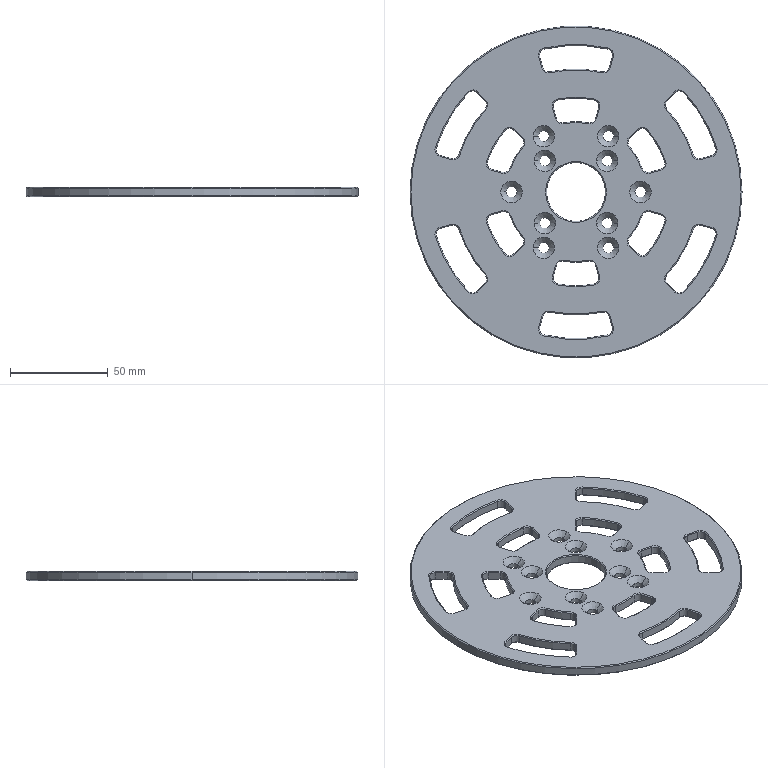Part | STEP file | 10000020546swp000-1 | 1 solid | 378 faces | box 170 x 170 x 5 mm | volume 86997 mm3 | cone 196 | cylinder 108 | plane 74 | commonest cylinder face diameters 6 x60 5.5 x20 72 x6 96 x6 126 x6 150 x6